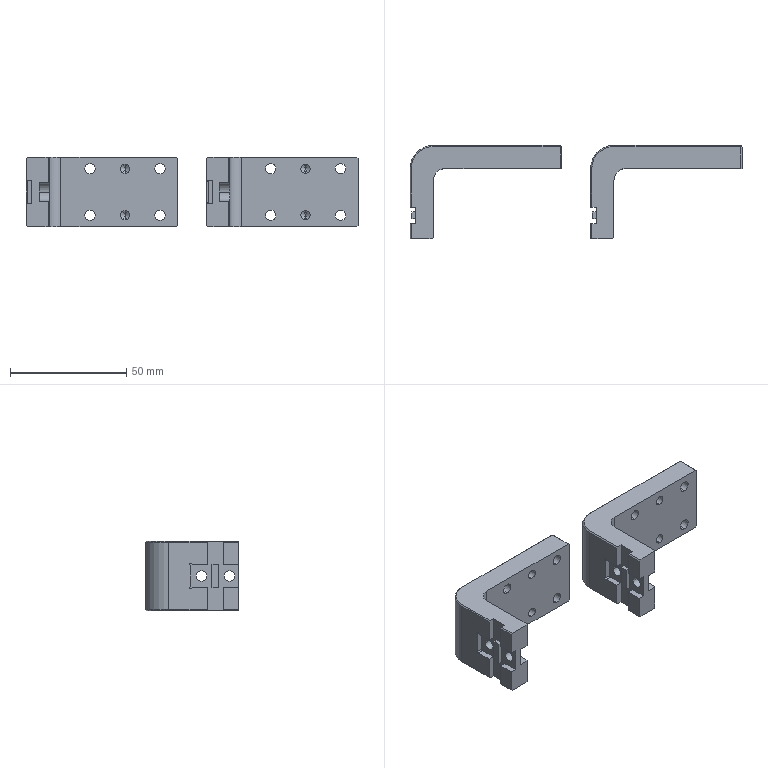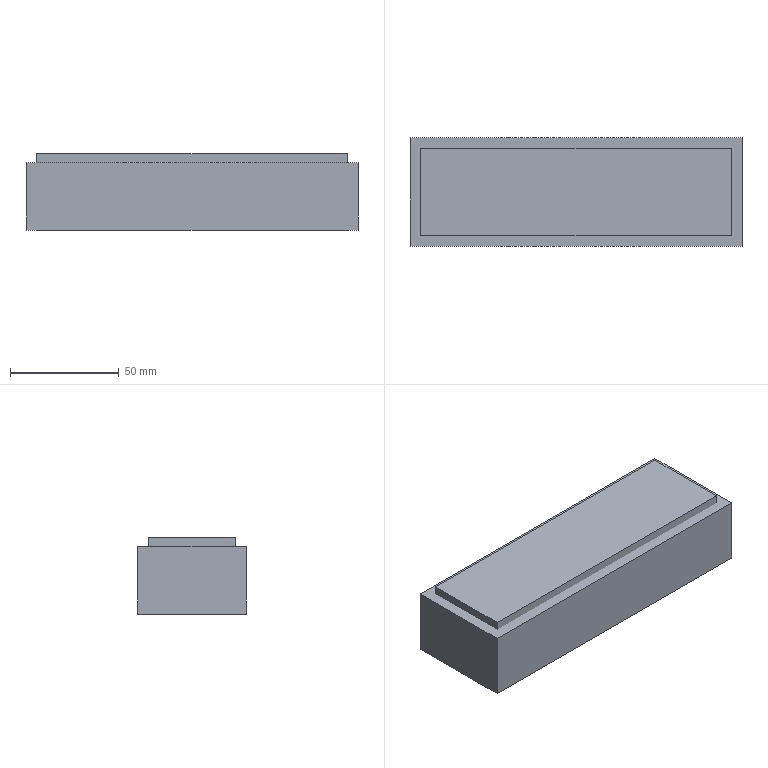CAM job | NX | 3+2 milling, drilling | part box 142.5 x 40 x 30 mm | stock box 152.5 x 50 x 35 mm
Tools:
number,name,description,diameter,corner_radius,flute_length,length,flutes
19,D80,Milling Tool-5 Parameters,80.0,0.0,50.0,75.0,2
15,D10,Milling Tool-5 Parameters,10.0,0.0,50.0,75.0,2
14,D10JING,Milling Tool-5 Parameters,10.0,0.0,50.0,75.0,2
1,D6A45,Milling Tool-5 Parameters,6.0,0.0,50.0,75.0,2
8,4.5ZT,Drilling Tool,4.5,0.0,35.0,50.0,2
12,D6,Milling Tool-5 Parameters,6.0,0.0,50.0,75.0,2
16,1.0ZT,Drilling Tool,1.0,0.0,35.0,50.0,2
17,D2,Milling Tool-5 Parameters,2.0,0.0,50.0,75.0,2
18,3.8ZT,Drilling Tool,3.8,0.0,35.0,50.0,2
Operations:
program,operation,operation_type,tool,method,geometry_group,spindle_rpm,surface_speed,feed_per_tooth,feed_cut,feed_plunge,cut_length_mm,path_length_mm,cut_time_min,machine_time_min
1,FLOOR_WALL,VolumeBased25DMillingOperation,D80,METHOD,A,6500.0,1633.0,0.1154,1500.0,100.0,244.5,298.5,0.163,0.1684
1,ADAPTIVE_MILLING,CavityMilling,D10,METHOD,A,9500.0,298.0,0.1842,3500.0,1000.0,20584.232,21658.314,5.892,5.999
1,ADAPTIVE_MILLING_COPY,CavityMilling,D10,METHOD,A,9500.0,298.0,0.1842,3500.0,1000.0,20596.291,21820.984,5.895,6.018
1,刀补14,ZLevelMilling,D10JING,METHOD,A,9500.0,298.0,0.0632,1200.0,1000.0,2042.252,2389.774,1.807,1.842
1,PLANAR_MILL_COPY_COPY_COPY,PlanarMilling,D6A45,METHOD,A,9500.0,179.0,0.0658,1250.0,100.0,435.633,629.401,0.3485,0.3679
2,DRILLING,Operation,D6A45,METHOD,B,5000.0,94.0,0.035,350.0,0.0,32.0,333.789,0.0914,0.1216
2,DRILLING_COPY_COPY_COPY_1,Operation,4.5ZT,METHOD,B,2000.0,26.0,0.075,300.0,0.0,122.816,515.42,0.4094,0.4486
2,HOLE_MILLING,CylinderMilling,D6,METHOD,B,9500.0,179.0,0.0789,1500.0,100.0,589.727,1290.027,0.3932,0.4632
2,PLANAR_MILL_COPY_COPY_COPY_COPY,PlanarMilling,D6A45,METHOD,B,9500.0,179.0,0.0658,1250.0,100.0,210.025,885.147,0.168,0.2355
3,FLOOR_WALL_COPY,VolumeBased25DMillingOperation,D80,METHOD,C,6500.0,1633.0,0.1154,1500.0,100.0,1172.5,2336.501,0.7817,0.8981
3,PLANAR_MILL_COPY_COPY_COPY_COPY_1,PlanarMilling,D6A45,METHOD,C,9500.0,179.0,0.0658,1250.0,100.0,435.633,629.401,0.3485,0.3679
4,DRILLING_COPY,Operation,D6A45,METHOD,D,5000.0,94.0,0.035,350.0,0.0,15.0,129.175,0.0429,0.0543
4,DRILLING_COPY_COPY_COPY_1_COPY,Operation,4.5ZT,METHOD,D,2000.0,26.0,0.075,300.0,0.0,30.704,136.777,0.1023,0.113
4,DRILLING_COPY_COPY_COPY_1_COPY_COPY,Operation,1.0ZT,METHOD,D,2000.0,6.0,0.02,80.0,0.0,11.601,96.642,0.145,0.1535
4,FLOOR_WALL_1,VolumeBased25DMillingOperation,D2,METHOD,D,9500.0,59.0,0.0658,1250.0,100.0,5945.639,11704.525,4.756,5.332
4,FLOOR_WALL_1_COPY,VolumeBased25DMillingOperation,D2,METHOD,D,9500.0,59.0,0.0658,1250.0,100.0,324.697,402.037,0.2598,0.2675
4,PLANAR_MILL_COPY_COPY_COPY_COPY_1_COPY,PlanarMilling,D6A45,METHOD,D,9500.0,179.0,0.0658,1250.0,100.0,223.789,452.167,0.179,0.2019
4,刀补17,VolumeBased25DMillingOperation,D2,METHOD,D,9500.0,59.0,0.0658,1250.0,100.0,138.308,212.609,0.1106,0.1181
5,HOLE_MILLING_1,CylinderMilling,D6,METHOD,E,5500.0,103.0,0.0455,500.0,100.0,71.195,245.095,0.1424,0.1598
5,ZLEVEL_PROFILE,ZLevelMilling,D6,METHOD,E,5000.0,94.0,0.05,500.0,100.0,286.812,474.157,0.5736,0.5924
6,DRILLING_COPY_COPY,Operation,D6A45,METHOD,F,5000.0,94.0,0.035,350.0,0.0,7.5,158.224,0.0214,0.0365
6,DRILLING_COPY_COPY_COPY_1_COPY_1,Operation,3.8ZT,METHOD,F,2000.0,26.0,0.075,300.0,0.0,24.283,191.79,0.0809,0.0977
6,PLANAR_MILL_COPY_COPY_COPY_COPY_1_COPY_COPY,PlanarMilling,D6A45,METHOD,F,9500.0,179.0,0.0658,1250.0,100.0,93.323,887.519,0.0747,0.1541
6,刀补11,CylinderMilling,D2,METHOD,F,9500.0,59.0,0.0789,1500.0,100.0,120.836,395.836,0.0806,0.1081